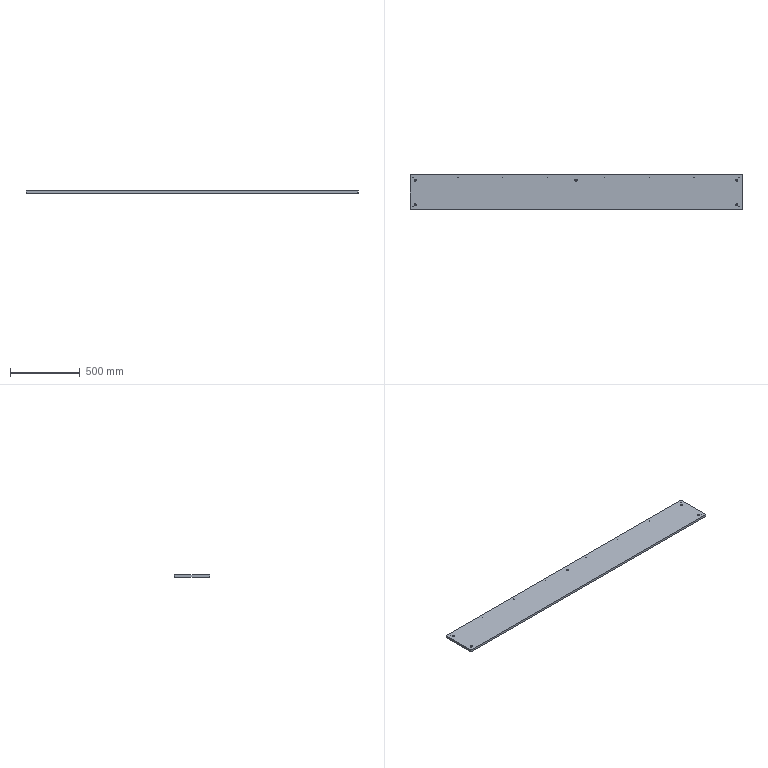Part | NX | features BREP 1 | 1 solid | 55 faces | box 2374 x 252 x 16 mm | volume 9560416 mm3 | cylinder 40 | plane 15 | commonest cylinder face diameters 3.3 x20 9 x10 15 x10